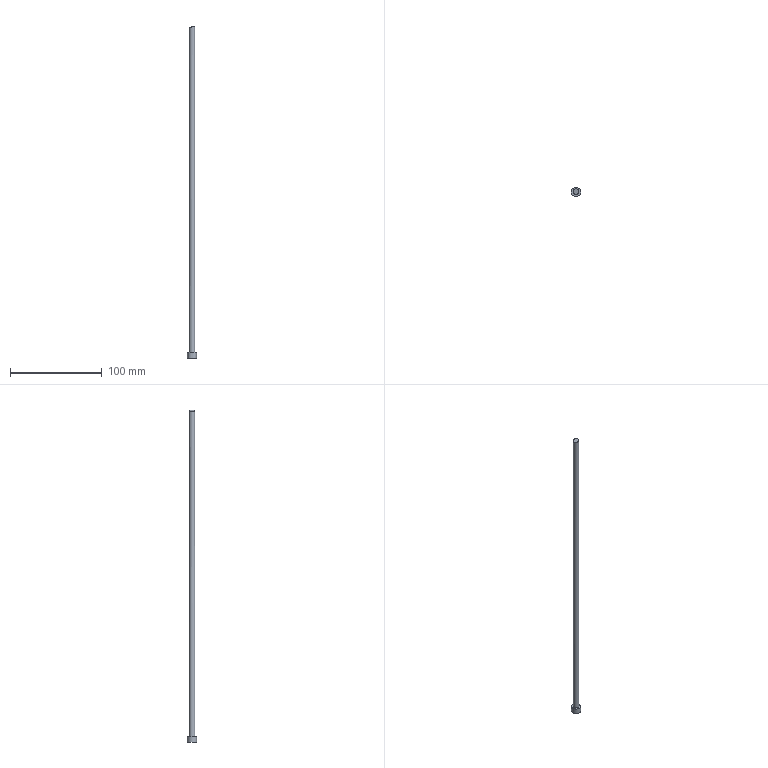Part | NX | features solid 2 | 1 solid | 5 faces | box 10 x 10 x 362.073 mm | volume 10509 mm3 | cylinder 2 | plane 2 | spline 1 | commonest cylinder face diameters 6 x1 10 x1
STEP:
#1=CARTESIAN_POINT('',(3.,69.,-339.5));
#2=VERTEX_POINT('',#1);
#3=CARTESIAN_POINT('',(0.,69.,-339.5));
#4=DIRECTION('',(0.,0.,1.));
#5=DIRECTION('',(1.,0.,0.));
#6=AXIS2_PLACEMENT_3D('',#3,#4,#5);
#7=CIRCLE('',#6,3.);
#8=EDGE_CURVE('',#2,#2,#7,.T.);
#9=ORIENTED_EDGE('',*,*,#8,.T.);
#10=EDGE_LOOP('',(#9));
#11=FACE_BOUND('',#10,.T.);
#12=CARTESIAN_POINT('',(-2.985,68.701,14.596));
#13=VERTEX_POINT('',#12);
#14=CARTESIAN_POINT('',(-2.061,66.403,14.965));
#15=CARTESIAN_POINT('',(-3.331,68.659,14.472));
#16=CARTESIAN_POINT('',(-2.527,71.169,14.721));
#17=CARTESIAN_POINT('',(-0.3082,72.287,15.471));
#18=CARTESIAN_POINT('',(2.059,71.604,16.246));
#19=CARTESIAN_POINT('',(3.33,69.342,16.667));
#20=CARTESIAN_POINT('',(2.532,66.831,16.464));
#21=CARTESIAN_POINT('',(0.2853,65.709,15.771));
#22=CARTESIAN_POINT('',(-2.061,66.403,14.965));
#23=CARTESIAN_POINT('',(-3.331,68.659,14.472));
#24=CARTESIAN_POINT('',(-2.527,71.169,14.721));
#25=B_SPLINE_CURVE_WITH_KNOTS('',3,(#14,#15,#16,#17,#18,#19,#20,#21,#22,#23,#24),.UNSPECIFIED.,.T.,.F.,(1,1,1,1,1,1,1,1,1,1,1,1,1,1,1),(-0.007227,-0.004818,-0.002409,0.,0.002409,0.004818,0.007227,0.009635,0.01204,0.01445,0.01686,0.01927,0.02168,0.02409,0.0265),.UNSPECIFIED.);
#26=EDGE_CURVE('',#13,#13,#25,.T.);
#27=ORIENTED_EDGE('',*,*,#26,.T.);
#28=EDGE_LOOP('',(#27));
#29=FACE_BOUND('',#28,.T.);
#30=CARTESIAN_POINT('',(0.,69.,-345.5));
#31=DIRECTION('',(0.,0.,1.));
#32=DIRECTION('',(1.,0.,0.));
#33=AXIS2_PLACEMENT_3D('',#30,#31,#32);
#34=CYLINDRICAL_SURFACE('',#33,3.);
#35=ADVANCED_FACE('',(#11,#29),#34,.T.);
#36=ORIENTED_EDGE('',*,*,#8,.F.);
#37=EDGE_LOOP('',(#36));
#38=FACE_BOUND('',#37,.T.);
#39=CARTESIAN_POINT('',(5.,69.,-339.5));
#40=VERTEX_POINT('',#39);
#41=CARTESIAN_POINT('',(0.,69.,-339.5));
#42=DIRECTION('',(0.,0.,-1.));
#43=DIRECTION('',(1.,0.,0.));
#44=AXIS2_PLACEMENT_3D('',#41,#42,#43);
#45=CIRCLE('',#44,5.);
#46=EDGE_CURVE('',#40,#40,#45,.T.);
#47=ORIENTED_EDGE('',*,*,#46,.F.);
#48=EDGE_LOOP('',(#47));
#49=FACE_BOUND('',#48,.T.);
#50=CARTESIAN_POINT('',(0.,69.,-339.5));
#51=DIRECTION('',(0.,0.,1.));
#52=DIRECTION('',(1.,0.,0.));
#53=AXIS2_PLACEMENT_3D('',#50,#51,#52);
#54=PLANE('',#53);
#55=ADVANCED_FACE('',(#38,#49),#54,.T.);
#56=CARTESIAN_POINT('',(5.,69.,-345.5));
#57=VERTEX_POINT('',#56);
#58=CARTESIAN_POINT('',(0.,69.,-345.5));
#59=DIRECTION('',(0.,0.,1.));
#60=DIRECTION('',(1.,0.,0.));
#61=AXIS2_PLACEMENT_3D('',#58,#59,#60);
#62=CIRCLE('',#61,5.);
#63=EDGE_CURVE('',#57,#57,#62,.T.);
#64=ORIENTED_EDGE('',*,*,#63,.F.);
#65=EDGE_LOOP('',(#64));
#66=FACE_BOUND('',#65,.T.);
#67=CARTESIAN_POINT('',(0.,69.,-345.5));
#68=DIRECTION('',(0.,0.,-1.));
#69=DIRECTION('',(-1.,0.,0.));
#70=AXIS2_PLACEMENT_3D('',#67,#68,#69);
#71=PLANE('',#70);
#72=ADVANCED_FACE('',(#66),#71,.T.);
#73=ORIENTED_EDGE('',*,*,#46,.T.);
#74=EDGE_LOOP('',(#73));
#75=FACE_BOUND('',#74,.T.);
#76=ORIENTED_EDGE('',*,*,#63,.T.);
#77=EDGE_LOOP('',(#76));
#78=FACE_BOUND('',#77,.T.);
#79=CARTESIAN_POINT('',(0.,69.,-345.5));
#80=DIRECTION('',(0.,0.,1.));
#81=DIRECTION('',(1.,0.,0.));
#82=AXIS2_PLACEMENT_3D('',#79,#80,#81);
#83=CYLINDRICAL_SURFACE('',#82,5.);
#84=ADVANCED_FACE('',(#75,#78),#83,.T.);
#85=ORIENTED_EDGE('',*,*,#26,.F.);
#86=EDGE_LOOP('',(#85));
#87=FACE_BOUND('',#86,.T.);
#88=CARTESIAN_POINT('',(-3.07,65.945,14.612));
#89=CARTESIAN_POINT('',(-3.059,67.979,14.581));
#90=CARTESIAN_POINT('',(-3.047,70.014,14.551));
#91=CARTESIAN_POINT('',(-3.035,72.048,14.524));
#92=CARTESIAN_POINT('',(-1.05,65.945,15.332));
#93=CARTESIAN_POINT('',(-1.04,67.98,15.302));
#94=CARTESIAN_POINT('',(-1.029,70.014,15.273));
#95=CARTESIAN_POINT('',(-1.017,72.049,15.245));
#96=CARTESIAN_POINT('',(0.9875,65.946,16.003));
#97=CARTESIAN_POINT('',(0.9975,67.981,15.974));
#98=CARTESIAN_POINT('',(1.008,70.015,15.945));
#99=CARTESIAN_POINT('',(1.019,72.05,15.918));
#100=CARTESIAN_POINT('',(3.04,65.947,16.632));
#101=CARTESIAN_POINT('',(3.049,67.981,16.602));
#102=CARTESIAN_POINT('',(3.059,70.016,16.574));
#103=CARTESIAN_POINT('',(3.07,72.051,16.548));
#104=B_SPLINE_SURFACE_WITH_KNOTS('',3,3,((#88,#89,#90,#91),(#92,#93,#94,#95),(#96,#97,#98,#99),(#100,#101,#102,#103)),.UNSPECIFIED.,.F.,.F.,.F.,(4,4),(4,4),(0.6292,0.6617),(0.8037,0.9196),.PIECEWISE_BEZIER_KNOTS.);
#105=ADVANCED_FACE('',(#87),#104,.T.);
#106=CLOSED_SHELL('',(#35,#55,#72,#84,#105));
#107=MANIFOLD_SOLID_BREP('',#106);
#108=(LENGTH_UNIT()NAMED_UNIT(*)SI_UNIT(.MILLI.,.METRE.));
#109=UNCERTAINTY_MEASURE_WITH_UNIT(LENGTH_MEASURE(0.0508),#108,'','');
#110=(NAMED_UNIT(*)PLANE_ANGLE_UNIT()SI_UNIT($,.RADIAN.));
#111=(NAMED_UNIT(*)SI_UNIT($,.STERADIAN.)SOLID_ANGLE_UNIT());
#112=(GEOMETRIC_REPRESENTATION_CONTEXT(3)GLOBAL_UNCERTAINTY_ASSIGNED_CONTEXT((#109))GLOBAL_UNIT_ASSIGNED_CONTEXT((#108,#110,#111))REPRESENTATION_CONTEXT('',''));
#113=ADVANCED_BREP_SHAPE_REPRESENTATION('',(#107),#112);